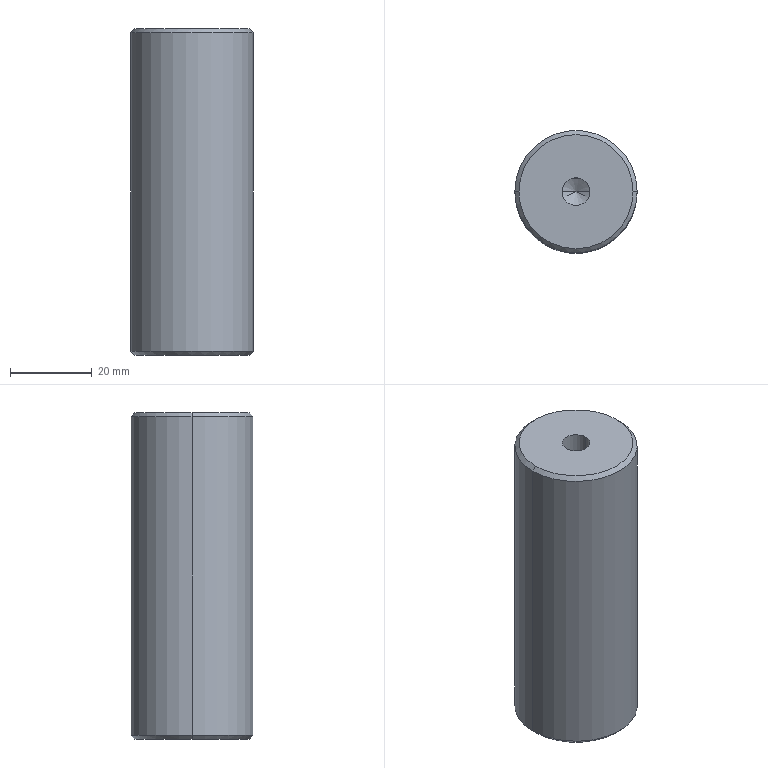Part | STEP file | SHAFT_DIA30_80V11 | 1 solid | 16 faces | box 30 x 30 x 80 mm | volume 54791 mm3 | cone 8 | cylinder 6 | plane 2 | commonest cylinder face diameters 6.8 x4 30 x2
STEP:
#1=CARTESIAN_POINT('',(0.,0.,0.));
#2=DIRECTION('',(0.,0.,1.));
#3=DIRECTION('',(1.,0.,0.));
#4=AXIS2_PLACEMENT_3D('',#1,#2,#3);
#5=CARTESIAN_POINT('',(-3.4,0.,22.25));
#6=VERTEX_POINT('',#5);
#7=CARTESIAN_POINT('',(-3.4,0.,0.));
#8=VERTEX_POINT('',#7);
#9=CARTESIAN_POINT('',(-3.4,0.,0.));
#10=DIRECTION('',(0.,0.,-1.));
#11=VECTOR('',#10,1.);
#12=LINE('',#9,#11);
#13=CARTESIAN_POINT('',(0.,0.,0.));
#14=DIRECTION('',(0.,0.,-1.));
#15=DIRECTION('',(-1.,0.,0.));
#16=AXIS2_PLACEMENT_3D('',#13,#14,#15);
#17=CYLINDRICAL_SURFACE('',#16,3.4);
#18=CARTESIAN_POINT('',(6.283,0.));
#19=DIRECTION('',(0.,1.));
#20=VECTOR('',#19,1.);
#21=LINE('',#18,#20);
#22=(GEOMETRIC_REPRESENTATION_CONTEXT(2)PARAMETRIC_REPRESENTATION_CONTEXT()REPRESENTATION_CONTEXT('',''));
#23=DEFINITIONAL_REPRESENTATION('',(#21),#22);
#24=PCURVE('',#17,#23);
#25=CARTESIAN_POINT('',(0.,0.,0.));
#26=DIRECTION('',(0.,0.,-1.));
#27=DIRECTION('',(-1.,0.,0.));
#28=AXIS2_PLACEMENT_3D('',#25,#26,#27);
#29=CYLINDRICAL_SURFACE('',#28,3.4);
#30=CARTESIAN_POINT('',(0.,0.));
#31=DIRECTION('',(0.,1.));
#32=VECTOR('',#31,1.);
#33=LINE('',#30,#32);
#34=(GEOMETRIC_REPRESENTATION_CONTEXT(2)PARAMETRIC_REPRESENTATION_CONTEXT()REPRESENTATION_CONTEXT('',''));
#35=DEFINITIONAL_REPRESENTATION('',(#33),#34);
#36=PCURVE('',#29,#35);
#37=SURFACE_CURVE('',#12,(#24,#36),.PCURVE_S1.);
#38=EDGE_CURVE('',#6,#8,#37,.T.);
#39=ORIENTED_EDGE('',*,*,#38,.T.);
#40=CARTESIAN_POINT('',(3.4,0.,0.));
#41=VERTEX_POINT('',#40);
#42=CARTESIAN_POINT('',(0.,0.,0.));
#43=DIRECTION('',(0.,0.,-1.));
#44=DIRECTION('',(-1.,0.,0.));
#45=AXIS2_PLACEMENT_3D('',#42,#43,#44);
#46=CIRCLE('',#45,3.4);
#47=CARTESIAN_POINT('',(0.,0.));
#48=DIRECTION('',(1.,0.));
#49=VECTOR('',#48,1.);
#50=LINE('',#47,#49);
#51=(GEOMETRIC_REPRESENTATION_CONTEXT(2)PARAMETRIC_REPRESENTATION_CONTEXT()REPRESENTATION_CONTEXT('',''));
#52=DEFINITIONAL_REPRESENTATION('',(#50),#51);
#53=PCURVE('',#17,#52);
#54=CARTESIAN_POINT('',(0.,0.,0.));
#55=DIRECTION('',(0.,0.,1.));
#56=DIRECTION('',(1.,0.,0.));
#57=AXIS2_PLACEMENT_3D('',#54,#55,#56);
#58=PLANE('',#57);
#59=CARTESIAN_POINT('',(-3.4,0.));
#60=CARTESIAN_POINT('',(-3.4,5.889));
#61=CARTESIAN_POINT('',(1.7,2.944));
#62=CARTESIAN_POINT('',(6.8,0.));
#63=CARTESIAN_POINT('',(1.7,-2.944));
#64=CARTESIAN_POINT('',(-3.4,-5.889));
#65=CARTESIAN_POINT('',(-3.4,0.));
#66=(BOUNDED_CURVE()B_SPLINE_CURVE(2,(#59,#60,#61,#62,#63,#64,#65),.UNSPECIFIED.,.T.,.F.)B_SPLINE_CURVE_WITH_KNOTS((1,2,2,2,2,1),(-2.094,0.,2.094,4.189,6.283,8.378),.UNSPECIFIED.)CURVE()GEOMETRIC_REPRESENTATION_ITEM()RATIONAL_B_SPLINE_CURVE((1.,0.5,1.,0.5,1.,0.5,1.))REPRESENTATION_ITEM(''));
#67=(GEOMETRIC_REPRESENTATION_CONTEXT(2)PARAMETRIC_REPRESENTATION_CONTEXT()REPRESENTATION_CONTEXT('',''));
#68=DEFINITIONAL_REPRESENTATION('',(#66),#67);
#69=PCURVE('',#58,#68);
#70=SURFACE_CURVE('',#46,(#53,#69),.PCURVE_S1.);
#71=EDGE_CURVE('',#41,#8,#70,.T.);
#72=ORIENTED_EDGE('',*,*,#71,.F.);
#73=CARTESIAN_POINT('',(3.4,0.,22.25));
#74=VERTEX_POINT('',#73);
#75=CARTESIAN_POINT('',(3.4,0.,0.));
#76=DIRECTION('',(0.,0.,-1.));
#77=VECTOR('',#76,1.);
#78=LINE('',#75,#77);
#79=CARTESIAN_POINT('',(3.142,0.));
#80=DIRECTION('',(0.,1.));
#81=VECTOR('',#80,1.);
#82=LINE('',#79,#81);
#83=(GEOMETRIC_REPRESENTATION_CONTEXT(2)PARAMETRIC_REPRESENTATION_CONTEXT()REPRESENTATION_CONTEXT('',''));
#84=DEFINITIONAL_REPRESENTATION('',(#82),#83);
#85=PCURVE('',#17,#84);
#86=CARTESIAN_POINT('',(3.142,0.));
#87=DIRECTION('',(0.,1.));
#88=VECTOR('',#87,1.);
#89=LINE('',#86,#88);
#90=(GEOMETRIC_REPRESENTATION_CONTEXT(2)PARAMETRIC_REPRESENTATION_CONTEXT()REPRESENTATION_CONTEXT('',''));
#91=DEFINITIONAL_REPRESENTATION('',(#89),#90);
#92=PCURVE('',#29,#91);
#93=SURFACE_CURVE('',#78,(#85,#92),.PCURVE_S1.);
#94=EDGE_CURVE('',#74,#41,#93,.T.);
#95=ORIENTED_EDGE('',*,*,#94,.F.);
#96=CARTESIAN_POINT('',(0.,0.,22.25));
#97=DIRECTION('',(0.,0.,-1.));
#98=DIRECTION('',(-1.,0.,0.));
#99=AXIS2_PLACEMENT_3D('',#96,#97,#98);
#100=CIRCLE('',#99,3.4);
#101=CARTESIAN_POINT('',(0.,-22.25));
#102=DIRECTION('',(1.,0.));
#103=VECTOR('',#102,1.);
#104=LINE('',#101,#103);
#105=(GEOMETRIC_REPRESENTATION_CONTEXT(2)PARAMETRIC_REPRESENTATION_CONTEXT()REPRESENTATION_CONTEXT('',''));
#106=DEFINITIONAL_REPRESENTATION('',(#104),#105);
#107=PCURVE('',#17,#106);
#108=CARTESIAN_POINT('',(0.,0.,22.25));
#109=DIRECTION('',(0.,0.,-1.));
#110=DIRECTION('',(-1.,0.,0.));
#111=AXIS2_PLACEMENT_3D('',#108,#109,#110);
#112=CONICAL_SURFACE('',#111,3.4,1.03);
#113=CARTESIAN_POINT('',(0.,0.));
#114=DIRECTION('',(1.,0.));
#115=VECTOR('',#114,1.);
#116=LINE('',#113,#115);
#117=(GEOMETRIC_REPRESENTATION_CONTEXT(2)PARAMETRIC_REPRESENTATION_CONTEXT()REPRESENTATION_CONTEXT('',''));
#118=DEFINITIONAL_REPRESENTATION('',(#116),#117);
#119=PCURVE('',#112,#118);
#120=SURFACE_CURVE('',#100,(#107,#119),.PCURVE_S1.);
#121=EDGE_CURVE('',#74,#6,#120,.T.);
#122=ORIENTED_EDGE('',*,*,#121,.T.);
#123=EDGE_LOOP('',(#39,#72,#95,#122));
#124=FACE_BOUND('',#123,.F.);
#125=ADVANCED_FACE('',(#124),#17,.F.);
#126=ORIENTED_EDGE('',*,*,#121,.F.);
#127=CARTESIAN_POINT('',(0.,0.,24.293));
#128=VERTEX_POINT('',#127);
#129=CARTESIAN_POINT('',(3.4,0.,22.25));
#130=DIRECTION('',(0.8572,0.,-0.515));
#131=VECTOR('',#130,1.);
#132=LINE('',#129,#131);
#133=CARTESIAN_POINT('',(3.142,-2.043));
#134=CARTESIAN_POINT('',(3.142,-2.012));
#135=CARTESIAN_POINT('',(3.142,-1.95));
#136=CARTESIAN_POINT('',(3.142,-1.857));
#137=CARTESIAN_POINT('',(3.142,-1.764));
#138=CARTESIAN_POINT('',(3.142,-1.671));
#139=CARTESIAN_POINT('',(3.142,-1.579));
#140=CARTESIAN_POINT('',(3.142,-1.486));
#141=CARTESIAN_POINT('',(3.142,-1.393));
#142=CARTESIAN_POINT('',(3.142,-1.3));
#143=CARTESIAN_POINT('',(3.142,-1.207));
#144=CARTESIAN_POINT('',(3.142,-1.114));
#145=CARTESIAN_POINT('',(3.142,-1.021));
#146=CARTESIAN_POINT('',(3.142,-0.9286));
#147=CARTESIAN_POINT('',(3.142,-0.8357));
#148=CARTESIAN_POINT('',(3.142,-0.7429));
#149=CARTESIAN_POINT('',(3.142,-0.65));
#150=CARTESIAN_POINT('',(3.142,-0.5572));
#151=CARTESIAN_POINT('',(3.142,-0.4643));
#152=CARTESIAN_POINT('',(3.142,-0.3714));
#153=CARTESIAN_POINT('',(3.142,-0.2786));
#154=CARTESIAN_POINT('',(3.142,-0.1857));
#155=CARTESIAN_POINT('',(3.142,-0.09286));
#156=CARTESIAN_POINT('',(3.142,-0.03095));
#157=CARTESIAN_POINT('',(3.142,0.));
#158=B_SPLINE_CURVE_WITH_KNOTS('',3,(#133,#134,#135,#136,#137,#138,#139,#140,#141,#142,#143,#144,#145,#146,#147,#148,#149,#150,#151,#152,#153,#154,#155,#156,#157),.UNSPECIFIED.,.F.,.F.,(4,1,1,1,1,1,1,1,1,1,1,1,1,1,1,1,1,1,1,1,1,1,4),(-3.967,-3.786,-3.606,-3.426,-3.245,-3.065,-2.885,-2.704,-2.524,-2.344,-2.164,-1.983,-1.803,-1.623,-1.442,-1.262,-1.082,-0.9015,-0.7212,-0.5409,-0.3606,-0.1803,0.),.QUASI_UNIFORM_KNOTS.);
#159=(GEOMETRIC_REPRESENTATION_CONTEXT(2)PARAMETRIC_REPRESENTATION_CONTEXT()REPRESENTATION_CONTEXT('',''));
#160=DEFINITIONAL_REPRESENTATION('',(#158),#159);
#161=PCURVE('',#112,#160);
#162=CARTESIAN_POINT('',(0.,0.,22.25));
#163=DIRECTION('',(0.,0.,-1.));
#164=DIRECTION('',(-1.,0.,0.));
#165=AXIS2_PLACEMENT_3D('',#162,#163,#164);
#166=CONICAL_SURFACE('',#165,3.4,1.03);
#167=CARTESIAN_POINT('',(3.142,-2.043));
#168=CARTESIAN_POINT('',(3.142,-2.012));
#169=CARTESIAN_POINT('',(3.142,-1.95));
#170=CARTESIAN_POINT('',(3.142,-1.857));
#171=CARTESIAN_POINT('',(3.142,-1.764));
#172=CARTESIAN_POINT('',(3.142,-1.671));
#173=CARTESIAN_POINT('',(3.142,-1.579));
#174=CARTESIAN_POINT('',(3.142,-1.486));
#175=CARTESIAN_POINT('',(3.142,-1.393));
#176=CARTESIAN_POINT('',(3.142,-1.3));
#177=CARTESIAN_POINT('',(3.142,-1.207));
#178=CARTESIAN_POINT('',(3.142,-1.114));
#179=CARTESIAN_POINT('',(3.142,-1.021));
#180=CARTESIAN_POINT('',(3.142,-0.9286));
#181=CARTESIAN_POINT('',(3.142,-0.8357));
#182=CARTESIAN_POINT('',(3.142,-0.7429));
#183=CARTESIAN_POINT('',(3.142,-0.65));
#184=CARTESIAN_POINT('',(3.142,-0.5572));
#185=CARTESIAN_POINT('',(3.142,-0.4643));
#186=CARTESIAN_POINT('',(3.142,-0.3714));
#187=CARTESIAN_POINT('',(3.142,-0.2786));
#188=CARTESIAN_POINT('',(3.142,-0.1857));
#189=CARTESIAN_POINT('',(3.142,-0.09286));
#190=CARTESIAN_POINT('',(3.142,-0.03095));
#191=CARTESIAN_POINT('',(3.142,0.));
#192=B_SPLINE_CURVE_WITH_KNOTS('',3,(#167,#168,#169,#170,#171,#172,#173,#174,#175,#176,#177,#178,#179,#180,#181,#182,#183,#184,#185,#186,#187,#188,#189,#190,#191),.UNSPECIFIED.,.F.,.F.,(4,1,1,1,1,1,1,1,1,1,1,1,1,1,1,1,1,1,1,1,1,1,4),(-3.967,-3.786,-3.606,-3.426,-3.245,-3.065,-2.885,-2.704,-2.524,-2.344,-2.164,-1.983,-1.803,-1.623,-1.442,-1.262,-1.082,-0.9015,-0.7212,-0.5409,-0.3606,-0.1803,0.),.QUASI_UNIFORM_KNOTS.);
#193=(GEOMETRIC_REPRESENTATION_CONTEXT(2)PARAMETRIC_REPRESENTATION_CONTEXT()REPRESENTATION_CONTEXT('',''));
#194=DEFINITIONAL_REPRESENTATION('',(#192),#193);
#195=PCURVE('',#166,#194);
#196=SURFACE_CURVE('',#132,(#161,#195),.PCURVE_S1.);
#197=EDGE_CURVE('',#128,#74,#196,.T.);
#198=ORIENTED_EDGE('',*,*,#197,.F.);
#199=CARTESIAN_POINT('',(-3.4,0.,22.25));
#200=DIRECTION('',(-0.8572,0.,-0.515));
#201=VECTOR('',#200,1.);
#202=LINE('',#199,#201);
#203=CARTESIAN_POINT('',(6.283,0.));
#204=DIRECTION('',(0.,1.));
#205=VECTOR('',#204,1.);
#206=LINE('',#203,#205);
#207=(GEOMETRIC_REPRESENTATION_CONTEXT(2)PARAMETRIC_REPRESENTATION_CONTEXT()REPRESENTATION_CONTEXT('',''));
#208=DEFINITIONAL_REPRESENTATION('',(#206),#207);
#209=PCURVE('',#112,#208);
#210=CARTESIAN_POINT('',(0.,0.));
#211=DIRECTION('',(0.,1.));
#212=VECTOR('',#211,1.);
#213=LINE('',#210,#212);
#214=(GEOMETRIC_REPRESENTATION_CONTEXT(2)PARAMETRIC_REPRESENTATION_CONTEXT()REPRESENTATION_CONTEXT('',''));
#215=DEFINITIONAL_REPRESENTATION('',(#213),#214);
#216=PCURVE('',#166,#215);
#217=SURFACE_CURVE('',#202,(#209,#216),.PCURVE_S1.);
#218=EDGE_CURVE('',#128,#6,#217,.T.);
#219=ORIENTED_EDGE('',*,*,#218,.T.);
#220=EDGE_LOOP('',(#126,#198,#219));
#221=FACE_BOUND('',#220,.F.);
#222=ADVANCED_FACE('',(#221),#112,.F.);
#223=CARTESIAN_POINT('',(3.4,0.,57.75));
#224=VERTEX_POINT('',#223);
#225=CARTESIAN_POINT('',(3.4,0.,80.));
#226=VERTEX_POINT('',#225);
#227=CARTESIAN_POINT('',(3.4,0.,80.));
#228=DIRECTION('',(0.,0.,1.));
#229=VECTOR('',#228,1.);
#230=LINE('',#227,#229);
#231=CARTESIAN_POINT('',(0.,0.,80.));
#232=DIRECTION('',(0.,0.,1.));
#233=DIRECTION('',(1.,0.,0.));
#234=AXIS2_PLACEMENT_3D('',#231,#232,#233);
#235=CYLINDRICAL_SURFACE('',#234,3.4);
#236=CARTESIAN_POINT('',(6.283,0.));
#237=DIRECTION('',(0.,1.));
#238=VECTOR('',#237,1.);
#239=LINE('',#236,#238);
#240=(GEOMETRIC_REPRESENTATION_CONTEXT(2)PARAMETRIC_REPRESENTATION_CONTEXT()REPRESENTATION_CONTEXT('',''));
#241=DEFINITIONAL_REPRESENTATION('',(#239),#240);
#242=PCURVE('',#235,#241);
#243=CARTESIAN_POINT('',(0.,0.,80.));
#244=DIRECTION('',(0.,0.,1.));
#245=DIRECTION('',(1.,0.,0.));
#246=AXIS2_PLACEMENT_3D('',#243,#244,#245);
#247=CYLINDRICAL_SURFACE('',#246,3.4);
#248=CARTESIAN_POINT('',(0.,0.));
#249=DIRECTION('',(0.,1.));
#250=VECTOR('',#249,1.);
#251=LINE('',#248,#250);
#252=(GEOMETRIC_REPRESENTATION_CONTEXT(2)PARAMETRIC_REPRESENTATION_CONTEXT()REPRESENTATION_CONTEXT('',''));
#253=DEFINITIONAL_REPRESENTATION('',(#251),#252);
#254=PCURVE('',#247,#253);
#255=SURFACE_CURVE('',#230,(#242,#254),.PCURVE_S1.);
#256=EDGE_CURVE('',#224,#226,#255,.T.);
#257=ORIENTED_EDGE('',*,*,#256,.T.);
#258=CARTESIAN_POINT('',(-3.4,0.,80.));
#259=VERTEX_POINT('',#258);
#260=CARTESIAN_POINT('',(0.,0.,80.));
#261=DIRECTION('',(0.,0.,1.));
#262=DIRECTION('',(1.,0.,0.));
#263=AXIS2_PLACEMENT_3D('',#260,#261,#262);
#264=CIRCLE('',#263,3.4);
#265=CARTESIAN_POINT('',(0.,0.));
#266=DIRECTION('',(1.,0.));
#267=VECTOR('',#266,1.);
#268=LINE('',#265,#267);
#269=(GEOMETRIC_REPRESENTATION_CONTEXT(2)PARAMETRIC_REPRESENTATION_CONTEXT()REPRESENTATION_CONTEXT('',''));
#270=DEFINITIONAL_REPRESENTATION('',(#268),#269);
#271=PCURVE('',#235,#270);
#272=CARTESIAN_POINT('',(0.,0.,80.));
#273=DIRECTION('',(0.,0.,1.));
#274=DIRECTION('',(1.,0.,0.));
#275=AXIS2_PLACEMENT_3D('',#272,#273,#274);
#276=PLANE('',#275);
#277=CARTESIAN_POINT('',(0.,0.));
#278=DIRECTION('',(1.,0.));
#279=AXIS2_PLACEMENT_2D('',#277,#278);
#280=CIRCLE('',#279,3.4);
#281=(GEOMETRIC_REPRESENTATION_CONTEXT(2)PARAMETRIC_REPRESENTATION_CONTEXT()REPRESENTATION_CONTEXT('',''));
#282=DEFINITIONAL_REPRESENTATION('',(#280),#281);
#283=PCURVE('',#276,#282);
#284=SURFACE_CURVE('',#264,(#271,#283),.PCURVE_S1.);
#285=EDGE_CURVE('',#259,#226,#284,.T.);
#286=ORIENTED_EDGE('',*,*,#285,.F.);
#287=CARTESIAN_POINT('',(-3.4,0.,57.75));
#288=VERTEX_POINT('',#287);
#289=CARTESIAN_POINT('',(-3.4,0.,80.));
#290=DIRECTION('',(0.,0.,1.));
#291=VECTOR('',#290,1.);
#292=LINE('',#289,#291);
#293=CARTESIAN_POINT('',(3.142,0.));
#294=DIRECTION('',(0.,1.));
#295=VECTOR('',#294,1.);
#296=LINE('',#293,#295);
#297=(GEOMETRIC_REPRESENTATION_CONTEXT(2)PARAMETRIC_REPRESENTATION_CONTEXT()REPRESENTATION_CONTEXT('',''));
#298=DEFINITIONAL_REPRESENTATION('',(#296),#297);
#299=PCURVE('',#235,#298);
#300=CARTESIAN_POINT('',(3.142,0.));
#301=DIRECTION('',(0.,1.));
#302=VECTOR('',#301,1.);
#303=LINE('',#300,#302);
#304=(GEOMETRIC_REPRESENTATION_CONTEXT(2)PARAMETRIC_REPRESENTATION_CONTEXT()REPRESENTATION_CONTEXT('',''));
#305=DEFINITIONAL_REPRESENTATION('',(#303),#304);
#306=PCURVE('',#247,#305);
#307=SURFACE_CURVE('',#292,(#299,#306),.PCURVE_S1.);
#308=EDGE_CURVE('',#288,#259,#307,.T.);
#309=ORIENTED_EDGE('',*,*,#308,.F.);
#310=CARTESIAN_POINT('',(0.,0.,57.75));
#311=DIRECTION('',(0.,0.,1.));
#312=DIRECTION('',(1.,0.,0.));
#313=AXIS2_PLACEMENT_3D('',#310,#311,#312);
#314=CIRCLE('',#313,3.4);
#315=CARTESIAN_POINT('',(0.,-22.25));
#316=DIRECTION('',(1.,0.));
#317=VECTOR('',#316,1.);
#318=LINE('',#315,#317);
#319=(GEOMETRIC_REPRESENTATION_CONTEXT(2)PARAMETRIC_REPRESENTATION_CONTEXT()REPRESENTATION_CONTEXT('',''));
#320=DEFINITIONAL_REPRESENTATION('',(#318),#319);
#321=PCURVE('',#235,#320);
#322=CARTESIAN_POINT('',(0.,0.,57.75));
#323=DIRECTION('',(0.,0.,1.));
#324=DIRECTION('',(1.,0.,0.));
#325=AXIS2_PLACEMENT_3D('',#322,#323,#324);
#326=CONICAL_SURFACE('',#325,3.4,1.03);
#327=CARTESIAN_POINT('',(0.,0.));
#328=DIRECTION('',(1.,0.));
#329=VECTOR('',#328,1.);
#330=LINE('',#327,#329);
#331=(GEOMETRIC_REPRESENTATION_CONTEXT(2)PARAMETRIC_REPRESENTATION_CONTEXT()REPRESENTATION_CONTEXT('',''));
#332=DEFINITIONAL_REPRESENTATION('',(#330),#331);
#333=PCURVE('',#326,#332);
#334=SURFACE_CURVE('',#314,(#321,#333),.PCURVE_S1.);
#335=EDGE_CURVE('',#288,#224,#334,.T.);
#336=ORIENTED_EDGE('',*,*,#335,.T.);
#337=EDGE_LOOP('',(#257,#286,#309,#336));
#338=FACE_BOUND('',#337,.F.);
#339=ADVANCED_FACE('',(#338),#235,.F.);
#340=ORIENTED_EDGE('',*,*,#335,.F.);
#341=CARTESIAN_POINT('',(0.,0.,55.707));
#342=VERTEX_POINT('',#341);
#343=CARTESIAN_POINT('',(-3.4,0.,57.75));
#344=DIRECTION('',(-0.8572,0.,0.515));
#345=VECTOR('',#344,1.);
#346=LINE('',#343,#345);
#347=CARTESIAN_POINT('',(3.142,0.));
#348=DIRECTION('',(0.,1.));
#349=VECTOR('',#348,1.);
#350=LINE('',#347,#349);
#351=(GEOMETRIC_REPRESENTATION_CONTEXT(2)PARAMETRIC_REPRESENTATION_CONTEXT()REPRESENTATION_CONTEXT('',''));
#352=DEFINITIONAL_REPRESENTATION('',(#350),#351);
#353=PCURVE('',#326,#352);
#354=CARTESIAN_POINT('',(0.,0.,57.75));
#355=DIRECTION('',(0.,0.,1.));
#356=DIRECTION('',(1.,0.,0.));
#357=AXIS2_PLACEMENT_3D('',#354,#355,#356);
#358=CONICAL_SURFACE('',#357,3.4,1.03);
#359=CARTESIAN_POINT('',(3.142,0.));
#360=DIRECTION('',(0.,1.));
#361=VECTOR('',#360,1.);
#362=LINE('',#359,#361);
#363=(GEOMETRIC_REPRESENTATION_CONTEXT(2)PARAMETRIC_REPRESENTATION_CONTEXT()REPRESENTATION_CONTEXT('',''));
#364=DEFINITIONAL_REPRESENTATION('',(#362),#363);
#365=PCURVE('',#358,#364);
#366=SURFACE_CURVE('',#346,(#353,#365),.PCURVE_S1.);
#367=EDGE_CURVE('',#342,#288,#366,.T.);
#368=ORIENTED_EDGE('',*,*,#367,.F.);
#369=CARTESIAN_POINT('',(3.4,0.,57.75));
#370=DIRECTION('',(0.8572,0.,0.515));
#371=VECTOR('',#370,1.);
#372=LINE('',#369,#371);
#373=CARTESIAN_POINT('',(6.283,0.));
#374=DIRECTION('',(0.,1.));
#375=VECTOR('',#374,1.);
#376=LINE('',#373,#375);
#377=(GEOMETRIC_REPRESENTATION_CONTEXT(2)PARAMETRIC_REPRESENTATION_CONTEXT()REPRESENTATION_CONTEXT('',''));
#378=DEFINITIONAL_REPRESENTATION('',(#376),#377);
#379=PCURVE('',#326,#378);
#380=CARTESIAN_POINT('',(0.,0.));
#381=DIRECTION('',(0.,1.));
#382=VECTOR('',#381,1.);
#383=LINE('',#380,#382);
#384=(GEOMETRIC_REPRESENTATION_CONTEXT(2)PARAMETRIC_REPRESENTATION_CONTEXT()REPRESENTATION_CONTEXT('',''));
#385=DEFINITIONAL_REPRESENTATION('',(#383),#384);
#386=PCURVE('',#358,#385);
#387=SURFACE_CURVE('',#372,(#379,#386),.PCURVE_S1.);
#388=EDGE_CURVE('',#342,#224,#387,.T.);
#389=ORIENTED_EDGE('',*,*,#388,.T.);
#390=EDGE_LOOP('',(#340,#368,#389));
#391=FACE_BOUND('',#390,.F.);
#392=ADVANCED_FACE('',(#391),#326,.F.);
#393=CARTESIAN_POINT('',(14.,0.,80.));
#394=VERTEX_POINT('',#393);
#395=CARTESIAN_POINT('',(-14.,0.,80.));
#396=VERTEX_POINT('',#395);
#397=CARTESIAN_POINT('',(0.,0.,80.));
#398=DIRECTION('',(0.,0.,1.));
#399=DIRECTION('',(1.,0.,0.));
#400=AXIS2_PLACEMENT_3D('',#397,#398,#399);
#401=CIRCLE('',#400,14.);
#402=CARTESIAN_POINT('',(0.,0.,80.));
#403=DIRECTION('',(0.,0.,-1.));
#404=DIRECTION('',(-1.,0.,0.));
#405=AXIS2_PLACEMENT_3D('',#402,#403,#404);
#406=CONICAL_SURFACE('',#405,14.,0.7854);
#407=CARTESIAN_POINT('',(3.142,0.));
#408=DIRECTION('',(-1.,0.));
#409=VECTOR('',#408,1.);
#410=LINE('',#407,#409);
#411=(GEOMETRIC_REPRESENTATION_CONTEXT(2)PARAMETRIC_REPRESENTATION_CONTEXT()REPRESENTATION_CONTEXT('',''));
#412=DEFINITIONAL_REPRESENTATION('',(#410),#411);
#413=PCURVE('',#406,#412);
#414=CARTESIAN_POINT('',(0.,0.));
#415=DIRECTION('',(1.,0.));
#416=AXIS2_PLACEMENT_2D('',#414,#415);
#417=CIRCLE('',#416,14.);
#418=(GEOMETRIC_REPRESENTATION_CONTEXT(2)PARAMETRIC_REPRESENTATION_CONTEXT()REPRESENTATION_CONTEXT('',''));
#419=DEFINITIONAL_REPRESENTATION('',(#417),#418);
#420=PCURVE('',#276,#419);
#421=SURFACE_CURVE('',#401,(#413,#420),.PCURVE_S1.);
#422=EDGE_CURVE('',#394,#396,#421,.T.);
#423=ORIENTED_EDGE('',*,*,#422,.F.);
#424=CARTESIAN_POINT('',(15.,0.,79.));
#425=VERTEX_POINT('',#424);
#426=CARTESIAN_POINT('',(14.,0.,80.));
#427=DIRECTION('',(0.7071,0.,-0.7071));
#428=VECTOR('',#427,1.);
#429=LINE('',#426,#428);
#430=CARTESIAN_POINT('',(3.142,0.));
#431=DIRECTION('',(0.,1.));
#432=VECTOR('',#431,1.);
#433=LINE('',#430,#432);
#434=(GEOMETRIC_REPRESENTATION_CONTEXT(2)PARAMETRIC_REPRESENTATION_CONTEXT()REPRESENTATION_CONTEXT('',''));
#435=DEFINITIONAL_REPRESENTATION('',(#433),#434);
#436=PCURVE('',#406,#435);
#437=CARTESIAN_POINT('',(0.,0.,80.));
#438=DIRECTION('',(0.,0.,-1.));
#439=DIRECTION('',(-1.,0.,0.));
#440=AXIS2_PLACEMENT_3D('',#437,#438,#439);
#441=CONICAL_SURFACE('',#440,14.,0.7854);
#442=CARTESIAN_POINT('',(3.142,0.));
#443=DIRECTION('',(0.,1.));
#444=VECTOR('',#443,1.);
#445=LINE('',#442,#444);
#446=(GEOMETRIC_REPRESENTATION_CONTEXT(2)PARAMETRIC_REPRESENTATION_CONTEXT()REPRESENTATION_CONTEXT('',''));
#447=DEFINITIONAL_REPRESENTATION('',(#445),#446);
#448=PCURVE('',#441,#447);
#449=SURFACE_CURVE('',#429,(#436,#448),.PCURVE_S1.);
#450=EDGE_CURVE('',#394,#425,#449,.T.);
#451=ORIENTED_EDGE('',*,*,#450,.T.);
#452=CARTESIAN_POINT('',(-15.,0.,79.));
#453=VERTEX_POINT('',#452);
#454=CARTESIAN_POINT('',(0.,0.,79.));
#455=DIRECTION('',(0.,0.,-1.));
#456=DIRECTION('',(1.,0.,0.));
#457=AXIS2_PLACEMENT_3D('',#454,#455,#456);
#458=CIRCLE('',#457,15.);
#459=CARTESIAN_POINT('',(-3.142,1.));
#460=DIRECTION('',(1.,0.));
#461=VECTOR('',#460,1.);
#462=LINE('',#459,#461);
#463=(GEOMETRIC_REPRESENTATION_CONTEXT(2)PARAMETRIC_REPRESENTATION_CONTEXT()REPRESENTATION_CONTEXT('',''));
#464=DEFINITIONAL_REPRESENTATION('',(#462),#463);
#465=PCURVE('',#406,#464);
#466=CARTESIAN_POINT('',(0.,0.,80.));
#467=DIRECTION('',(0.,0.,-1.));
#468=DIRECTION('',(-1.,0.,0.));
#469=AXIS2_PLACEMENT_3D('',#466,#467,#468);
#470=CYLINDRICAL_SURFACE('',#469,15.);
#471=CARTESIAN_POINT('',(-3.142,1.));
#472=DIRECTION('',(1.,0.));
#473=VECTOR('',#472,1.);
#474=LINE('',#471,#473);
#475=(GEOMETRIC_REPRESENTATION_CONTEXT(2)PARAMETRIC_REPRESENTATION_CONTEXT()REPRESENTATION_CONTEXT('',''));
#476=DEFINITIONAL_REPRESENTATION('',(#474),#475);
#477=PCURVE('',#470,#476);
#478=SURFACE_CURVE('',#458,(#465,#477),.PCURVE_S1.);
#479=EDGE_CURVE('',#453,#425,#478,.T.);
#480=ORIENTED_EDGE('',*,*,#479,.F.);
#481=CARTESIAN_POINT('',(-14.,0.,80.));
#482=DIRECTION('',(-0.7071,0.,-0.7071));
#483=VECTOR('',#482,1.);
#484=LINE('',#481,#483);
#485=CARTESIAN_POINT('',(0.,0.));
#486=DIRECTION('',(0.,1.));
#487=VECTOR('',#486,1.);
#488=LINE('',#485,#487);
#489=(GEOMETRIC_REPRESENTATION_CONTEXT(2)PARAMETRIC_REPRESENTATION_CONTEXT()REPRESENTATION_CONTEXT('',''));
#490=DEFINITIONAL_REPRESENTATION('',(#488),#489);
#491=PCURVE('',#406,#490);
#492=CARTESIAN_POINT('',(6.283,0.));
#493=DIRECTION('',(0.,1.));
#494=VECTOR('',#493,1.);
#495=LINE('',#492,#494);
#496=(GEOMETRIC_REPRESENTATION_CONTEXT(2)PARAMETRIC_REPRESENTATION_CONTEXT()REPRESENTATION_CONTEXT('',''));
#497=DEFINITIONAL_REPRESENTATION('',(#495),#496);
#498=PCURVE('',#441,#497);
#499=SURFACE_CURVE('',#484,(#491,#498),.PCURVE_S1.);
#500=EDGE_CURVE('',#396,#453,#499,.T.);
#501=ORIENTED_EDGE('',*,*,#500,.F.);
#502=EDGE_LOOP('',(#423,#451,#480,#501));
#503=FACE_BOUND('',#502,.T.);
#504=ADVANCED_FACE('',(#503),#406,.T.);
#505=CARTESIAN_POINT('',(-14.,0.,0.));
#506=VERTEX_POINT('',#505);
#507=CARTESIAN_POINT('',(14.,0.,0.));
#508=VERTEX_POINT('',#507);
#509=CARTESIAN_POINT('',(0.,0.,0.));
#510=DIRECTION('',(0.,0.,-1.));
#511=DIRECTION('',(1.,0.,0.));
#512=AXIS2_PLACEMENT_3D('',#509,#510,#511);
#513=CIRCLE('',#512,14.);
#514=CARTESIAN_POINT('',(0.,0.,1.));
#515=DIRECTION('',(0.,0.,1.));
#516=DIRECTION('',(1.,0.,0.));
#517=AXIS2_PLACEMENT_3D('',#514,#515,#516);
#518=CONICAL_SURFACE('',#517,15.,0.7854);
#519=CARTESIAN_POINT('',(6.283,-1.));
#520=DIRECTION('',(-1.,0.));
#521=VECTOR('',#520,1.);
#522=LINE('',#519,#521);
#523=(GEOMETRIC_REPRESENTATION_CONTEXT(2)PARAMETRIC_REPRESENTATION_CONTEXT()REPRESENTATION_CONTEXT('',''));
#524=DEFINITIONAL_REPRESENTATION('',(#522),#523);
#525=PCURVE('',#518,#524);
#526=CARTESIAN_POINT('',(14.,0.));
#527=CARTESIAN_POINT('',(14.,-24.249));
#528=CARTESIAN_POINT('',(-7.,-12.124));
#529=CARTESIAN_POINT('',(-28.,0.));
#530=CARTESIAN_POINT('',(-7.,12.124));
#531=CARTESIAN_POINT('',(14.,24.249));
#532=CARTESIAN_POINT('',(14.,0.));
#533=(BOUNDED_CURVE()B_SPLINE_CURVE(2,(#526,#527,#528,#529,#530,#531,#532),.UNSPECIFIED.,.T.,.F.)B_SPLINE_CURVE_WITH_KNOTS((1,2,2,2,2,1),(-2.094,0.,2.094,4.189,6.283,8.378),.UNSPECIFIED.)CURVE()GEOMETRIC_REPRESENTATION_ITEM()RATIONAL_B_SPLINE_CURVE((1.,0.5,1.,0.5,1.,0.5,1.))REPRESENTATION_ITEM(''));
#534=(GEOMETRIC_REPRESENTATION_CONTEXT(2)PARAMETRIC_REPRESENTATION_CONTEXT()REPRESENTATION_CONTEXT('',''));
#535=DEFINITIONAL_REPRESENTATION('',(#533),#534);
#536=PCURVE('',#58,#535);
#537=SURFACE_CURVE('',#513,(#525,#536),.PCURVE_S1.);
#538=EDGE_CURVE('',#506,#508,#537,.T.);
#539=ORIENTED_EDGE('',*,*,#538,.F.);
#540=CARTESIAN_POINT('',(-15.,0.,1.));
#541=VERTEX_POINT('',#540);
#542=CARTESIAN_POINT('',(-15.,0.,1.));
#543=DIRECTION('',(-0.7071,0.,0.7071));
#544=VECTOR('',#543,1.);
#545=LINE('',#542,#544);
#546=CARTESIAN_POINT('',(3.142,0.));
#547=DIRECTION('',(0.,1.));
#548=VECTOR('',#547,1.);
#549=LINE('',#546,#548);
#550=(GEOMETRIC_REPRESENTATION_CONTEXT(2)PARAMETRIC_REPRESENTATION_CONTEXT()REPRESENTATION_CONTEXT('',''));
#551=DEFINITIONAL_REPRESENTATION('',(#549),#550);
#552=PCURVE('',#518,#551);
#553=CARTESIAN_POINT('',(0.,0.,1.));
#554=DIRECTION('',(0.,0.,1.));
#555=DIRECTION('',(1.,0.,0.));
#556=AXIS2_PLACEMENT_3D('',#553,#554,#555);
#557=CONICAL_SURFACE('',#556,15.,0.7854);
#558=CARTESIAN_POINT('',(3.142,0.));
#559=DIRECTION('',(0.,1.));
#560=VECTOR('',#559,1.);
#561=LINE('',#558,#560);
#562=(GEOMETRIC_REPRESENTATION_CONTEXT(2)PARAMETRIC_REPRESENTATION_CONTEXT()REPRESENTATION_CONTEXT('',''));
#563=DEFINITIONAL_REPRESENTATION('',(#561),#562);
#564=PCURVE('',#557,#563);
#565=SURFACE_CURVE('',#545,(#552,#564),.PCURVE_S1.);
#566=EDGE_CURVE('',#506,#541,#565,.T.);
#567=ORIENTED_EDGE('',*,*,#566,.T.);
#568=CARTESIAN_POINT('',(15.,0.,1.));
#569=VERTEX_POINT('',#568);
#570=CARTESIAN_POINT('',(0.,0.,1.));
#571=DIRECTION('',(0.,0.,1.));
#572=DIRECTION('',(1.,0.,0.));
#573=AXIS2_PLACEMENT_3D('',#570,#571,#572);
#574=CIRCLE('',#573,15.);
#575=CARTESIAN_POINT('',(0.,0.));
#576=DIRECTION('',(1.,0.));
#577=VECTOR('',#576,1.);
#578=LINE('',#575,#577);
#579=(GEOMETRIC_REPRESENTATION_CONTEXT(2)PARAMETRIC_REPRESENTATION_CONTEXT()REPRESENTATION_CONTEXT('',''));
#580=DEFINITIONAL_REPRESENTATION('',(#578),#579);
#581=PCURVE('',#518,#580);
#582=CARTESIAN_POINT('',(3.142,79.));
#583=DIRECTION('',(-1.,0.));
#584=VECTOR('',#583,1.);
#585=LINE('',#582,#584);
#586=(GEOMETRIC_REPRESENTATION_CONTEXT(2)PARAMETRIC_REPRESENTATION_CONTEXT()REPRESENTATION_CONTEXT('',''));
#587=DEFINITIONAL_REPRESENTATION('',(#585),#586);
#588=PCURVE('',#470,#587);
#589=SURFACE_CURVE('',#574,(#581,#588),.PCURVE_S1.);
#590=EDGE_CURVE('',#569,#541,#589,.T.);
#591=ORIENTED_EDGE('',*,*,#590,.F.);
#592=CARTESIAN_POINT('',(15.,0.,1.));
#593=DIRECTION('',(0.7071,0.,0.7071));
#594=VECTOR('',#593,1.);
#595=LINE('',#592,#594);
#596=CARTESIAN_POINT('',(0.,0.));
#597=DIRECTION('',(0.,1.));
#598=VECTOR('',#597,1.);
#599=LINE('',#596,#598);
#600=(GEOMETRIC_REPRESENTATION_CONTEXT(2)PARAMETRIC_REPRESENTATION_CONTEXT()REPRESENTATION_CONTEXT('',''));
#601=DEFINITIONAL_REPRESENTATION('',(#599),#600);
#602=PCURVE('',#518,#601);
#603=CARTESIAN_POINT('',(6.283,0.));
#604=DIRECTION('',(0.,1.));
#605=VECTOR('',#604,1.);
#606=LINE('',#603,#605);
#607=(GEOMETRIC_REPRESENTATION_CONTEXT(2)PARAMETRIC_REPRESENTATION_CONTEXT()REPRESENTATION_CONTEXT('',''));
#608=DEFINITIONAL_REPRESENTATION('',(#606),#607);
#609=PCURVE('',#557,#608);
#610=SURFACE_CURVE('',#595,(#602,#609),.PCURVE_S1.);
#611=EDGE_CURVE('',#508,#569,#610,.T.);
#612=ORIENTED_EDGE('',*,*,#611,.F.);
#613=EDGE_LOOP('',(#539,#567,#591,#612));
#614=FACE_BOUND('',#613,.T.);
#615=ADVANCED_FACE('',(#614),#518,.T.);
#616=ORIENTED_EDGE('',*,*,#479,.T.);
#617=CARTESIAN_POINT('',(15.,0.,80.));
#618=DIRECTION('',(0.,0.,-1.));
#619=VECTOR('',#618,1.);
#620=LINE('',#617,#619);
#621=CARTESIAN_POINT('',(3.142,0.));
#622=DIRECTION('',(0.,1.));
#623=VECTOR('',#622,1.);
#624=LINE('',#621,#623);
#625=(GEOMETRIC_REPRESENTATION_CONTEXT(2)PARAMETRIC_REPRESENTATION_CONTEXT()REPRESENTATION_CONTEXT('',''));
#626=DEFINITIONAL_REPRESENTATION('',(#624),#625);
#627=PCURVE('',#470,#626);
#628=CARTESIAN_POINT('',(0.,0.,80.));
#629=DIRECTION('',(0.,0.,-1.));
#630=DIRECTION('',(-1.,0.,0.));
#631=AXIS2_PLACEMENT_3D('',#628,#629,#630);
#632=CYLINDRICAL_SURFACE('',#631,15.);
#633=CARTESIAN_POINT('',(3.142,0.));
#634=DIRECTION('',(0.,1.));
#635=VECTOR('',#634,1.);
#636=LINE('',#633,#635);
#637=(GEOMETRIC_REPRESENTATION_CONTEXT(2)PARAMETRIC_REPRESENTATION_CONTEXT()REPRESENTATION_CONTEXT('',''));
#638=DEFINITIONAL_REPRESENTATION('',(#636),#637);
#639=PCURVE('',#632,#638);
#640=SURFACE_CURVE('',#620,(#627,#639),.PCURVE_S1.);
#641=EDGE_CURVE('',#425,#569,#640,.T.);
#642=ORIENTED_EDGE('',*,*,#641,.T.);
#643=ORIENTED_EDGE('',*,*,#590,.T.);
#644=CARTESIAN_POINT('',(-15.,0.,80.));
#645=DIRECTION('',(0.,0.,-1.));
#646=VECTOR('',#645,1.);
#647=LINE('',#644,#646);
#648=CARTESIAN_POINT('',(0.,0.));
#649=DIRECTION('',(0.,1.));
#650=VECTOR('',#649,1.);
#651=LINE('',#648,#650);
#652=(GEOMETRIC_REPRESENTATION_CONTEXT(2)PARAMETRIC_REPRESENTATION_CONTEXT()REPRESENTATION_CONTEXT('',''));
#653=DEFINITIONAL_REPRESENTATION('',(#651),#652);
#654=PCURVE('',#470,#653);
#655=CARTESIAN_POINT('',(6.283,0.));
#656=DIRECTION('',(0.,1.));
#657=VECTOR('',#656,1.);
#658=LINE('',#655,#657);
#659=(GEOMETRIC_REPRESENTATION_CONTEXT(2)PARAMETRIC_REPRESENTATION_CONTEXT()REPRESENTATION_CONTEXT('',''));
#660=DEFINITIONAL_REPRESENTATION('',(#658),#659);
#661=PCURVE('',#632,#660);
#662=SURFACE_CURVE('',#647,(#654,#661),.PCURVE_S1.);
#663=EDGE_CURVE('',#453,#541,#662,.T.);
#664=ORIENTED_EDGE('',*,*,#663,.F.);
#665=EDGE_LOOP('',(#616,#642,#643,#664));
#666=FACE_BOUND('',#665,.T.);
#667=ADVANCED_FACE('',(#666),#470,.T.);
#668=ORIENTED_EDGE('',*,*,#641,.F.);
#669=CARTESIAN_POINT('',(0.,0.,79.));
#670=DIRECTION('',(0.,0.,-1.));
#671=DIRECTION('',(1.,0.,0.));
#672=AXIS2_PLACEMENT_3D('',#669,#670,#671);
#673=CIRCLE('',#672,15.);
#674=CARTESIAN_POINT('',(3.142,1.));
#675=DIRECTION('',(1.,0.));
#676=VECTOR('',#675,1.);
#677=LINE('',#674,#676);
#678=(GEOMETRIC_REPRESENTATION_CONTEXT(2)PARAMETRIC_REPRESENTATION_CONTEXT()REPRESENTATION_CONTEXT('',''));
#679=DEFINITIONAL_REPRESENTATION('',(#677),#678);
#680=PCURVE('',#632,#679);
#681=CARTESIAN_POINT('',(3.142,1.));
#682=DIRECTION('',(1.,0.));
#683=VECTOR('',#682,1.);
#684=LINE('',#681,#683);
#685=(GEOMETRIC_REPRESENTATION_CONTEXT(2)PARAMETRIC_REPRESENTATION_CONTEXT()REPRESENTATION_CONTEXT('',''));
#686=DEFINITIONAL_REPRESENTATION('',(#684),#685);
#687=PCURVE('',#441,#686);
#688=SURFACE_CURVE('',#673,(#680,#687),.PCURVE_S1.);
#689=EDGE_CURVE('',#425,#453,#688,.T.);
#690=ORIENTED_EDGE('',*,*,#689,.T.);
#691=ORIENTED_EDGE('',*,*,#663,.T.);
#692=CARTESIAN_POINT('',(0.,0.,1.));
#693=DIRECTION('',(0.,0.,1.));
#694=DIRECTION('',(1.,0.,0.));
#695=AXIS2_PLACEMENT_3D('',#692,#693,#694);
#696=CIRCLE('',#695,15.);
#697=CARTESIAN_POINT('',(9.425,79.));
#698=DIRECTION('',(-1.,0.));
#699=VECTOR('',#698,1.);
#700=LINE('',#697,#699);
#701=(GEOMETRIC_REPRESENTATION_CONTEXT(2)PARAMETRIC_REPRESENTATION_CONTEXT()REPRESENTATION_CONTEXT('',''));
#702=DEFINITIONAL_REPRESENTATION('',(#700),#701);
#703=PCURVE('',#632,#702);
#704=CARTESIAN_POINT('',(0.,0.));
#705=DIRECTION('',(1.,0.));
#706=VECTOR('',#705,1.);
#707=LINE('',#704,#706);
#708=(GEOMETRIC_REPRESENTATION_CONTEXT(2)PARAMETRIC_REPRESENTATION_CONTEXT()REPRESENTATION_CONTEXT('',''));
#709=DEFINITIONAL_REPRESENTATION('',(#707),#708);
#710=PCURVE('',#557,#709);
#711=SURFACE_CURVE('',#696,(#703,#710),.PCURVE_S1.);
#712=EDGE_CURVE('',#541,#569,#711,.T.);
#713=ORIENTED_EDGE('',*,*,#712,.T.);
#714=EDGE_LOOP('',(#668,#690,#691,#713));
#715=FACE_BOUND('',#714,.T.);
#716=ADVANCED_FACE('',(#715),#632,.T.);
#717=CARTESIAN_POINT('',(0.,0.,80.));
#718=DIRECTION('',(0.,0.,1.));
#719=DIRECTION('',(1.,0.,0.));
#720=AXIS2_PLACEMENT_3D('',#717,#718,#719);
#721=CIRCLE('',#720,3.4);
#722=CARTESIAN_POINT('',(0.,0.));
#723=DIRECTION('',(1.,0.));
#724=AXIS2_PLACEMENT_2D('',#722,#723);
#725=CIRCLE('',#724,3.4);
#726=(GEOMETRIC_REPRESENTATION_CONTEXT(2)PARAMETRIC_REPRESENTATION_CONTEXT()REPRESENTATION_CONTEXT('',''));
#727=DEFINITIONAL_REPRESENTATION('',(#725),#726);
#728=PCURVE('',#276,#727);
#729=CARTESIAN_POINT('',(0.,0.));
#730=DIRECTION('',(1.,0.));
#731=VECTOR('',#730,1.);
#732=LINE('',#729,#731);
#733=(GEOMETRIC_REPRESENTATION_CONTEXT(2)PARAMETRIC_REPRESENTATION_CONTEXT()REPRESENTATION_CONTEXT('',''));
#734=DEFINITIONAL_REPRESENTATION('',(#732),#733);
#735=PCURVE('',#247,#734);
#736=SURFACE_CURVE('',#721,(#728,#735),.PCURVE_S1.);
#737=EDGE_CURVE('',#226,#259,#736,.T.);
#738=ORIENTED_EDGE('',*,*,#737,.F.);
#739=ORIENTED_EDGE('',*,*,#285,.F.);
#740=EDGE_LOOP('',(#738,#739));
#741=FACE_BOUND('',#740,.T.);
#742=CARTESIAN_POINT('',(0.,0.,80.));
#743=DIRECTION('',(0.,0.,1.));
#744=DIRECTION('',(1.,0.,0.));
#745=AXIS2_PLACEMENT_3D('',#742,#743,#744);
#746=CIRCLE('',#745,14.);
#747=CARTESIAN_POINT('',(0.,0.));
#748=DIRECTION('',(1.,0.));
#749=AXIS2_PLACEMENT_2D('',#747,#748);
#750=CIRCLE('',#749,14.);
#751=(GEOMETRIC_REPRESENTATION_CONTEXT(2)PARAMETRIC_REPRESENTATION_CONTEXT()REPRESENTATION_CONTEXT('',''));
#752=DEFINITIONAL_REPRESENTATION('',(#750),#751);
#753=PCURVE('',#276,#752);
#754=CARTESIAN_POINT('',(9.425,0.));
#755=DIRECTION('',(-1.,0.));
#756=VECTOR('',#755,1.);
#757=LINE('',#754,#756);
#758=(GEOMETRIC_REPRESENTATION_CONTEXT(2)PARAMETRIC_REPRESENTATION_CONTEXT()REPRESENTATION_CONTEXT('',''));
#759=DEFINITIONAL_REPRESENTATION('',(#757),#758);
#760=PCURVE('',#441,#759);
#761=SURFACE_CURVE('',#746,(#753,#760),.PCURVE_S1.);
#762=EDGE_CURVE('',#396,#394,#761,.T.);
#763=ORIENTED_EDGE('',*,*,#762,.T.);
#764=ORIENTED_EDGE('',*,*,#422,.T.);
#765=EDGE_LOOP('',(#763,#764));
#766=FACE_BOUND('',#765,.T.);
#767=ADVANCED_FACE('',(#741,#766),#276,.T.);
#768=CARTESIAN_POINT('',(0.,0.,0.));
#769=DIRECTION('',(0.,0.,-1.));
#770=DIRECTION('',(-1.,0.,0.));
#771=AXIS2_PLACEMENT_3D('',#768,#769,#770);
#772=CIRCLE('',#771,3.4);
#773=CARTESIAN_POINT('',(-3.4,0.));
#774=CARTESIAN_POINT('',(-3.4,5.889));
#775=CARTESIAN_POINT('',(1.7,2.944));
#776=CARTESIAN_POINT('',(6.8,0.));
#777=CARTESIAN_POINT('',(1.7,-2.944));
#778=CARTESIAN_POINT('',(-3.4,-5.889));
#779=CARTESIAN_POINT('',(-3.4,0.));
#780=(BOUNDED_CURVE()B_SPLINE_CURVE(2,(#773,#774,#775,#776,#777,#778,#779),.UNSPECIFIED.,.T.,.F.)B_SPLINE_CURVE_WITH_KNOTS((1,2,2,2,2,1),(-2.094,0.,2.094,4.189,6.283,8.378),.UNSPECIFIED.)CURVE()GEOMETRIC_REPRESENTATION_ITEM()RATIONAL_B_SPLINE_CURVE((1.,0.5,1.,0.5,1.,0.5,1.))REPRESENTATION_ITEM(''));
#781=(GEOMETRIC_REPRESENTATION_CONTEXT(2)PARAMETRIC_REPRESENTATION_CONTEXT()REPRESENTATION_CONTEXT('',''));
#782=DEFINITIONAL_REPRESENTATION('',(#780),#781);
#783=PCURVE('',#58,#782);
#784=CARTESIAN_POINT('',(0.,0.));
#785=DIRECTION('',(1.,0.));
#786=VECTOR('',#785,1.);
#787=LINE('',#784,#786);
#788=(GEOMETRIC_REPRESENTATION_CONTEXT(2)PARAMETRIC_REPRESENTATION_CONTEXT()REPRESENTATION_CONTEXT('',''));
#789=DEFINITIONAL_REPRESENTATION('',(#787),#788);
#790=PCURVE('',#29,#789);
#791=SURFACE_CURVE('',#772,(#783,#790),.PCURVE_S1.);
#792=EDGE_CURVE('',#8,#41,#791,.T.);
#793=ORIENTED_EDGE('',*,*,#792,.F.);
#794=ORIENTED_EDGE('',*,*,#71,.F.);
#795=EDGE_LOOP('',(#793,#794));
#796=FACE_BOUND('',#795,.T.);
#797=CARTESIAN_POINT('',(0.,0.,0.));
#798=DIRECTION('',(0.,0.,-1.));
#799=DIRECTION('',(1.,0.,0.));
#800=AXIS2_PLACEMENT_3D('',#797,#798,#799);
#801=CIRCLE('',#800,14.);
#802=CARTESIAN_POINT('',(14.,0.));
#803=CARTESIAN_POINT('',(14.,-24.249));
#804=CARTESIAN_POINT('',(-7.,-12.124));
#805=CARTESIAN_POINT('',(-28.,0.));
#806=CARTESIAN_POINT('',(-7.,12.124));
#807=CARTESIAN_POINT('',(14.,24.249));
#808=CARTESIAN_POINT('',(14.,0.));
#809=(BOUNDED_CURVE()B_SPLINE_CURVE(2,(#802,#803,#804,#805,#806,#807,#808),.UNSPECIFIED.,.T.,.F.)B_SPLINE_CURVE_WITH_KNOTS((1,2,2,2,2,1),(-2.094,0.,2.094,4.189,6.283,8.378),.UNSPECIFIED.)CURVE()GEOMETRIC_REPRESENTATION_ITEM()RATIONAL_B_SPLINE_CURVE((1.,0.5,1.,0.5,1.,0.5,1.))REPRESENTATION_ITEM(''));
#810=(GEOMETRIC_REPRESENTATION_CONTEXT(2)PARAMETRIC_REPRESENTATION_CONTEXT()REPRESENTATION_CONTEXT('',''));
#811=DEFINITIONAL_REPRESENTATION('',(#809),#810);
#812=PCURVE('',#58,#811);
#813=CARTESIAN_POINT('',(6.283,-1.));
#814=DIRECTION('',(-1.,0.));
#815=VECTOR('',#814,1.);
#816=LINE('',#813,#815);
#817=(GEOMETRIC_REPRESENTATION_CONTEXT(2)PARAMETRIC_REPRESENTATION_CONTEXT()REPRESENTATION_CONTEXT('',''));
#818=DEFINITIONAL_REPRESENTATION('',(#816),#817);
#819=PCURVE('',#557,#818);
#820=SURFACE_CURVE('',#801,(#812,#819),.PCURVE_S1.);
#821=EDGE_CURVE('',#508,#506,#820,.T.);
#822=ORIENTED_EDGE('',*,*,#821,.T.);
#823=ORIENTED_EDGE('',*,*,#538,.T.);
#824=EDGE_LOOP('',(#822,#823));
#825=FACE_BOUND('',#824,.T.);
#826=ADVANCED_FACE('',(#796,#825),#58,.F.);
#827=ORIENTED_EDGE('',*,*,#566,.F.);
#828=ORIENTED_EDGE('',*,*,#821,.F.);
#829=ORIENTED_EDGE('',*,*,#611,.T.);
#830=ORIENTED_EDGE('',*,*,#712,.F.);
#831=EDGE_LOOP('',(#827,#828,#829,#830));
#832=FACE_BOUND('',#831,.T.);
#833=ADVANCED_FACE('',(#832),#557,.T.);
#834=ORIENTED_EDGE('',*,*,#450,.F.);
#835=ORIENTED_EDGE('',*,*,#762,.F.);
#836=ORIENTED_EDGE('',*,*,#500,.T.);
#837=ORIENTED_EDGE('',*,*,#689,.F.);
#838=EDGE_LOOP('',(#834,#835,#836,#837));
#839=FACE_BOUND('',#838,.T.);
#840=ADVANCED_FACE('',(#839),#441,.T.);
#841=CARTESIAN_POINT('',(0.,0.,57.75));
#842=DIRECTION('',(0.,0.,1.));
#843=DIRECTION('',(1.,0.,0.));
#844=AXIS2_PLACEMENT_3D('',#841,#842,#843);
#845=CIRCLE('',#844,3.4);
#846=CARTESIAN_POINT('',(0.,0.));
#847=DIRECTION('',(1.,0.));
#848=VECTOR('',#847,1.);
#849=LINE('',#846,#848);
#850=(GEOMETRIC_REPRESENTATION_CONTEXT(2)PARAMETRIC_REPRESENTATION_CONTEXT()REPRESENTATION_CONTEXT('',''));
#851=DEFINITIONAL_REPRESENTATION('',(#849),#850);
#852=PCURVE('',#358,#851);
#853=CARTESIAN_POINT('',(0.,-22.25));
#854=DIRECTION('',(1.,0.));
#855=VECTOR('',#854,1.);
#856=LINE('',#853,#855);
#857=(GEOMETRIC_REPRESENTATION_CONTEXT(2)PARAMETRIC_REPRESENTATION_CONTEXT()REPRESENTATION_CONTEXT('',''));
#858=DEFINITIONAL_REPRESENTATION('',(#856),#857);
#859=PCURVE('',#247,#858);
#860=SURFACE_CURVE('',#845,(#852,#859),.PCURVE_S1.);
#861=EDGE_CURVE('',#224,#288,#860,.T.);
#862=ORIENTED_EDGE('',*,*,#861,.F.);
#863=ORIENTED_EDGE('',*,*,#388,.F.);
#864=ORIENTED_EDGE('',*,*,#367,.T.);
#865=EDGE_LOOP('',(#862,#863,#864));
#866=FACE_BOUND('',#865,.F.);
#867=ADVANCED_FACE('',(#866),#358,.F.);
#868=ORIENTED_EDGE('',*,*,#737,.F.);
#869=ORIENTED_EDGE('',*,*,#256,.F.);
#870=ORIENTED_EDGE('',*,*,#861,.T.);
#871=ORIENTED_EDGE('',*,*,#308,.T.);
#872=EDGE_LOOP('',(#868,#869,#870,#871));
#873=FACE_BOUND('',#872,.F.);
#874=ADVANCED_FACE('',(#873),#247,.F.);
#875=CARTESIAN_POINT('',(0.,0.,22.25));
#876=DIRECTION('',(0.,0.,-1.));
#877=DIRECTION('',(-1.,0.,0.));
#878=AXIS2_PLACEMENT_3D('',#875,#876,#877);
#879=CIRCLE('',#878,3.4);
#880=CARTESIAN_POINT('',(0.,0.));
#881=DIRECTION('',(1.,0.));
#882=VECTOR('',#881,1.);
#883=LINE('',#880,#882);
#884=(GEOMETRIC_REPRESENTATION_CONTEXT(2)PARAMETRIC_REPRESENTATION_CONTEXT()REPRESENTATION_CONTEXT('',''));
#885=DEFINITIONAL_REPRESENTATION('',(#883),#884);
#886=PCURVE('',#166,#885);
#887=CARTESIAN_POINT('',(0.,-22.25));
#888=DIRECTION('',(1.,0.));
#889=VECTOR('',#888,1.);
#890=LINE('',#887,#889);
#891=(GEOMETRIC_REPRESENTATION_CONTEXT(2)PARAMETRIC_REPRESENTATION_CONTEXT()REPRESENTATION_CONTEXT('',''));
#892=DEFINITIONAL_REPRESENTATION('',(#890),#891);
#893=PCURVE('',#29,#892);
#894=SURFACE_CURVE('',#879,(#886,#893),.PCURVE_S1.);
#895=EDGE_CURVE('',#6,#74,#894,.T.);
#896=ORIENTED_EDGE('',*,*,#895,.F.);
#897=ORIENTED_EDGE('',*,*,#218,.F.);
#898=ORIENTED_EDGE('',*,*,#197,.T.);
#899=EDGE_LOOP('',(#896,#897,#898));
#900=FACE_BOUND('',#899,.F.);
#901=ADVANCED_FACE('',(#900),#166,.F.);
#902=ORIENTED_EDGE('',*,*,#792,.F.);
#903=ORIENTED_EDGE('',*,*,#38,.F.);
#904=ORIENTED_EDGE('',*,*,#895,.T.);
#905=ORIENTED_EDGE('',*,*,#94,.T.);
#906=EDGE_LOOP('',(#902,#903,#904,#905));
#907=FACE_BOUND('',#906,.F.);
#908=ADVANCED_FACE('',(#907),#29,.F.);
#909=CLOSED_SHELL('',(#125,#222,#339,#392,#504,#615,#667,#716,#767,#826,#833,#840,#867,#874,#901,#908));
#910=MANIFOLD_SOLID_BREP('',#909);
#911=(LENGTH_UNIT()NAMED_UNIT(*)SI_UNIT(.MILLI.,.METRE.));
#912=UNCERTAINTY_MEASURE_WITH_UNIT(LENGTH_MEASURE(0.0000001),#911,'','');
#913=(NAMED_UNIT(*)PLANE_ANGLE_UNIT()SI_UNIT($,.RADIAN.));
#914=(NAMED_UNIT(*)SI_UNIT($,.STERADIAN.)SOLID_ANGLE_UNIT());
#915=(GEOMETRIC_REPRESENTATION_CONTEXT(3)GLOBAL_UNCERTAINTY_ASSIGNED_CONTEXT((#912))GLOBAL_UNIT_ASSIGNED_CONTEXT((#911,#913,#914))REPRESENTATION_CONTEXT('',''));
#916=ADVANCED_BREP_SHAPE_REPRESENTATION('',(#4,#910),#915);